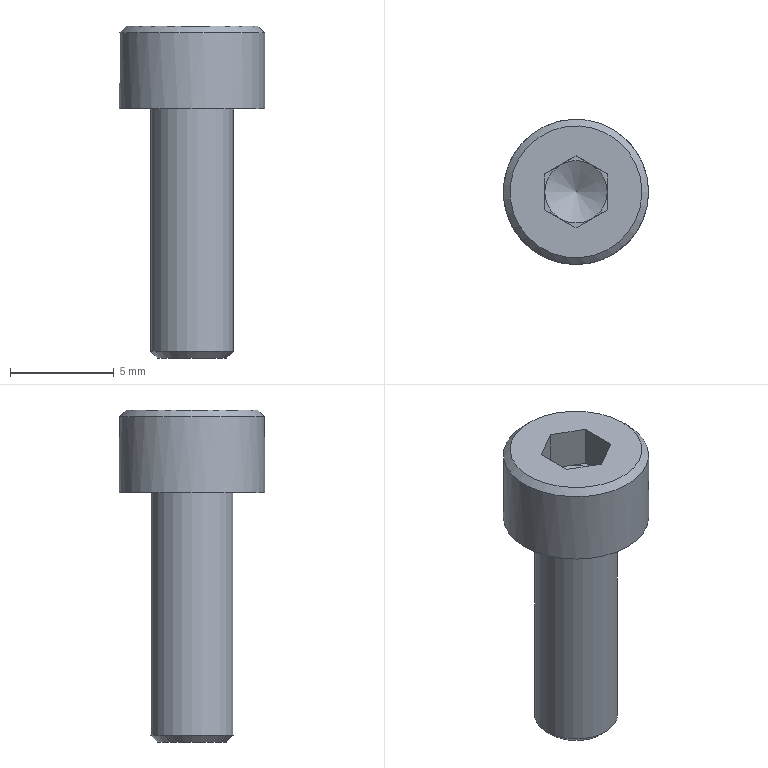Part | NX | features 切除-拉伸1 2 | 1 solid | 20 faces | box 7 x 7 x 16 mm | volume 285.405 mm3 | plane 15 | cone 3 | cylinder 2 | commonest cylinder face diameters 4 x1 7 x1
STEP:
#1=CARTESIAN_POINT('',(60.25,89.299,-85.1));
#2=VERTEX_POINT('',#1);
#3=CARTESIAN_POINT('',(59.5,88.,-85.1));
#4=VERTEX_POINT('',#3);
#5=CARTESIAN_POINT('',(61.,88.,-85.1));
#6=DIRECTION('',(0.,0.,1.));
#7=DIRECTION('',(-1.,0.,0.));
#8=AXIS2_PLACEMENT_3D('',#5,#6,#7);
#9=CIRCLE('',#8,1.5);
#10=EDGE_CURVE('',#2,#4,#9,.T.);
#11=ORIENTED_EDGE('',*,*,#10,.T.);
#12=CARTESIAN_POINT('',(60.25,86.701,-85.1));
#13=VERTEX_POINT('',#12);
#14=CARTESIAN_POINT('',(61.,88.,-85.1));
#15=DIRECTION('',(0.,0.,1.));
#16=DIRECTION('',(-1.,0.,0.));
#17=AXIS2_PLACEMENT_3D('',#14,#15,#16);
#18=CIRCLE('',#17,1.5);
#19=EDGE_CURVE('',#4,#13,#18,.T.);
#20=ORIENTED_EDGE('',*,*,#19,.T.);
#21=CARTESIAN_POINT('',(61.75,86.701,-85.1));
#22=VERTEX_POINT('',#21);
#23=CARTESIAN_POINT('',(61.,88.,-85.1));
#24=DIRECTION('',(0.,0.,1.));
#25=DIRECTION('',(-1.,0.,0.));
#26=AXIS2_PLACEMENT_3D('',#23,#24,#25);
#27=CIRCLE('',#26,1.5);
#28=EDGE_CURVE('',#13,#22,#27,.T.);
#29=ORIENTED_EDGE('',*,*,#28,.T.);
#30=CARTESIAN_POINT('',(62.5,88.,-85.1));
#31=VERTEX_POINT('',#30);
#32=CARTESIAN_POINT('',(61.,88.,-85.1));
#33=DIRECTION('',(0.,0.,1.));
#34=DIRECTION('',(-1.,0.,0.));
#35=AXIS2_PLACEMENT_3D('',#32,#33,#34);
#36=CIRCLE('',#35,1.5);
#37=EDGE_CURVE('',#22,#31,#36,.T.);
#38=ORIENTED_EDGE('',*,*,#37,.T.);
#39=CARTESIAN_POINT('',(61.75,89.299,-85.1));
#40=VERTEX_POINT('',#39);
#41=CARTESIAN_POINT('',(61.,88.,-85.1));
#42=DIRECTION('',(0.,0.,1.));
#43=DIRECTION('',(-1.,0.,0.));
#44=AXIS2_PLACEMENT_3D('',#41,#42,#43);
#45=CIRCLE('',#44,1.5);
#46=EDGE_CURVE('',#31,#40,#45,.T.);
#47=ORIENTED_EDGE('',*,*,#46,.T.);
#48=CARTESIAN_POINT('',(61.,88.,-85.1));
#49=DIRECTION('',(0.,0.,1.));
#50=DIRECTION('',(-1.,0.,0.));
#51=AXIS2_PLACEMENT_3D('',#48,#49,#50);
#52=CIRCLE('',#51,1.5);
#53=EDGE_CURVE('',#40,#2,#52,.T.);
#54=ORIENTED_EDGE('',*,*,#53,.T.);
#55=EDGE_LOOP('',(#11,#20,#29,#38,#47,#54));
#56=FACE_BOUND('',#55,.T.);
#57=CARTESIAN_POINT('',(61.,88.,-85.966));
#58=VERTEX_POINT('',#57);
#59=VERTEX_LOOP('',#58);
#60=FACE_BOUND('',#59,.T.);
#61=CARTESIAN_POINT('',(61.,88.,-85.1));
#62=DIRECTION('',(0.,0.,1.));
#63=DIRECTION('',(1.,0.,0.));
#64=AXIS2_PLACEMENT_3D('',#61,#62,#63);
#65=CONICAL_SURFACE('',#64,1.5,1.047);
#66=ADVANCED_FACE('',(#56,#60),#65,.F.);
#67=CARTESIAN_POINT('',(64.5,88.,-83.42));
#68=VERTEX_POINT('',#67);
#69=CARTESIAN_POINT('',(61.,88.,-83.42));
#70=DIRECTION('',(0.,0.,-1.));
#71=DIRECTION('',(1.,0.,0.));
#72=AXIS2_PLACEMENT_3D('',#69,#70,#71);
#73=CIRCLE('',#72,3.5);
#74=EDGE_CURVE('',#68,#68,#73,.T.);
#75=ORIENTED_EDGE('',*,*,#74,.F.);
#76=EDGE_LOOP('',(#75));
#77=FACE_BOUND('',#76,.T.);
#78=CARTESIAN_POINT('',(64.18,88.,-83.1));
#79=VERTEX_POINT('',#78);
#80=CARTESIAN_POINT('',(61.,88.,-83.1));
#81=DIRECTION('',(0.,0.,1.));
#82=DIRECTION('',(1.,0.,0.));
#83=AXIS2_PLACEMENT_3D('',#80,#81,#82);
#84=CIRCLE('',#83,3.18);
#85=EDGE_CURVE('',#79,#79,#84,.T.);
#86=ORIENTED_EDGE('',*,*,#85,.F.);
#87=EDGE_LOOP('',(#86));
#88=FACE_BOUND('',#87,.T.);
#89=CARTESIAN_POINT('',(61.,88.,-83.1));
#90=DIRECTION('',(0.,0.,-1.));
#91=DIRECTION('',(-1.,0.,0.));
#92=AXIS2_PLACEMENT_3D('',#89,#90,#91);
#93=CONICAL_SURFACE('',#92,3.18,0.7854);
#94=ADVANCED_FACE('',(#77,#88),#93,.T.);
#95=CARTESIAN_POINT('',(59.,88.,-98.78));
#96=VERTEX_POINT('',#95);
#97=CARTESIAN_POINT('',(61.,88.,-98.78));
#98=DIRECTION('',(0.,0.,1.));
#99=DIRECTION('',(-1.,0.,0.));
#100=AXIS2_PLACEMENT_3D('',#97,#98,#99);
#101=CIRCLE('',#100,2.);
#102=EDGE_CURVE('',#96,#96,#101,.T.);
#103=ORIENTED_EDGE('',*,*,#102,.F.);
#104=EDGE_LOOP('',(#103));
#105=FACE_BOUND('',#104,.T.);
#106=CARTESIAN_POINT('',(59.32,88.,-99.1));
#107=VERTEX_POINT('',#106);
#108=CARTESIAN_POINT('',(61.,88.,-99.1));
#109=DIRECTION('',(0.,0.,-1.));
#110=DIRECTION('',(-1.,0.,0.));
#111=AXIS2_PLACEMENT_3D('',#108,#109,#110);
#112=CIRCLE('',#111,1.68);
#113=EDGE_CURVE('',#107,#107,#112,.T.);
#114=ORIENTED_EDGE('',*,*,#113,.F.);
#115=EDGE_LOOP('',(#114));
#116=FACE_BOUND('',#115,.T.);
#117=CARTESIAN_POINT('',(61.,88.,-98.78));
#118=DIRECTION('',(0.,0.,1.));
#119=DIRECTION('',(1.,0.,0.));
#120=AXIS2_PLACEMENT_3D('',#117,#118,#119);
#121=CONICAL_SURFACE('',#120,2.,0.7854);
#122=ADVANCED_FACE('',(#105,#116),#121,.T.);
#123=CARTESIAN_POINT('',(59.,88.,-87.1));
#124=VERTEX_POINT('',#123);
#125=CARTESIAN_POINT('',(61.,88.,-87.1));
#126=DIRECTION('',(0.,0.,1.));
#127=DIRECTION('',(-1.,0.,0.));
#128=AXIS2_PLACEMENT_3D('',#125,#126,#127);
#129=CIRCLE('',#128,2.);
#130=EDGE_CURVE('',#124,#124,#129,.T.);
#131=ORIENTED_EDGE('',*,*,#130,.F.);
#132=EDGE_LOOP('',(#131));
#133=FACE_BOUND('',#132,.T.);
#134=ORIENTED_EDGE('',*,*,#102,.T.);
#135=EDGE_LOOP('',(#134));
#136=FACE_BOUND('',#135,.T.);
#137=CARTESIAN_POINT('',(61.,88.,-79.35));
#138=DIRECTION('',(0.,0.,1.));
#139=DIRECTION('',(1.,0.,0.));
#140=AXIS2_PLACEMENT_3D('',#137,#138,#139);
#141=CYLINDRICAL_SURFACE('',#140,2.);
#142=ADVANCED_FACE('',(#133,#136),#141,.T.);
#143=ORIENTED_EDGE('',*,*,#74,.T.);
#144=EDGE_LOOP('',(#143));
#145=FACE_BOUND('',#144,.T.);
#146=CARTESIAN_POINT('',(57.5,88.,-87.1));
#147=VERTEX_POINT('',#146);
#148=CARTESIAN_POINT('',(61.,88.,-87.1));
#149=DIRECTION('',(0.,0.,1.));
#150=DIRECTION('',(-1.,0.,0.));
#151=AXIS2_PLACEMENT_3D('',#148,#149,#150);
#152=CIRCLE('',#151,3.5);
#153=EDGE_CURVE('',#147,#147,#152,.T.);
#154=ORIENTED_EDGE('',*,*,#153,.T.);
#155=EDGE_LOOP('',(#154));
#156=FACE_BOUND('',#155,.T.);
#157=CARTESIAN_POINT('',(61.,88.,-79.35));
#158=DIRECTION('',(0.,0.,1.));
#159=DIRECTION('',(1.,0.,0.));
#160=AXIS2_PLACEMENT_3D('',#157,#158,#159);
#161=CYLINDRICAL_SURFACE('',#160,3.5);
#162=ADVANCED_FACE('',(#145,#156),#161,.T.);
#163=ORIENTED_EDGE('',*,*,#85,.T.);
#164=EDGE_LOOP('',(#163));
#165=FACE_BOUND('',#164,.T.);
#166=CARTESIAN_POINT('',(62.5,87.134,-83.1));
#167=VERTEX_POINT('',#166);
#168=CARTESIAN_POINT('',(61.,86.268,-83.1));
#169=VERTEX_POINT('',#168);
#170=CARTESIAN_POINT('',(62.875,87.35,-83.1));
#171=DIRECTION('',(-0.866,-0.5,0.));
#172=VECTOR('',#171,1000.);
#173=LINE('',#170,#172);
#174=EDGE_CURVE('',#167,#169,#173,.T.);
#175=ORIENTED_EDGE('',*,*,#174,.T.);
#176=CARTESIAN_POINT('',(59.5,87.134,-83.1));
#177=VERTEX_POINT('',#176);
#178=CARTESIAN_POINT('',(61.375,86.051,-83.1));
#179=DIRECTION('',(-0.866,0.5,0.));
#180=VECTOR('',#179,1000.);
#181=LINE('',#178,#180);
#182=EDGE_CURVE('',#169,#177,#181,.T.);
#183=ORIENTED_EDGE('',*,*,#182,.T.);
#184=CARTESIAN_POINT('',(59.5,88.866,-83.1));
#185=VERTEX_POINT('',#184);
#186=CARTESIAN_POINT('',(59.5,88.,-83.1));
#187=DIRECTION('',(0.,1.,0.));
#188=VECTOR('',#187,1000.);
#189=LINE('',#186,#188);
#190=EDGE_CURVE('',#177,#185,#189,.T.);
#191=ORIENTED_EDGE('',*,*,#190,.T.);
#192=CARTESIAN_POINT('',(61.,89.732,-83.1));
#193=VERTEX_POINT('',#192);
#194=CARTESIAN_POINT('',(61.375,89.949,-83.1));
#195=DIRECTION('',(0.866,0.5,0.));
#196=VECTOR('',#195,1000.);
#197=LINE('',#194,#196);
#198=EDGE_CURVE('',#185,#193,#197,.T.);
#199=ORIENTED_EDGE('',*,*,#198,.T.);
#200=CARTESIAN_POINT('',(62.5,88.866,-83.1));
#201=VERTEX_POINT('',#200);
#202=CARTESIAN_POINT('',(62.875,88.65,-83.1));
#203=DIRECTION('',(0.866,-0.5,0.));
#204=VECTOR('',#203,1000.);
#205=LINE('',#202,#204);
#206=EDGE_CURVE('',#193,#201,#205,.T.);
#207=ORIENTED_EDGE('',*,*,#206,.T.);
#208=CARTESIAN_POINT('',(62.5,88.,-83.1));
#209=DIRECTION('',(0.,-1.,0.));
#210=VECTOR('',#209,1000.);
#211=LINE('',#208,#210);
#212=EDGE_CURVE('',#201,#167,#211,.T.);
#213=ORIENTED_EDGE('',*,*,#212,.T.);
#214=EDGE_LOOP('',(#175,#183,#191,#199,#207,#213));
#215=FACE_BOUND('',#214,.T.);
#216=CARTESIAN_POINT('',(62.5,88.,-83.1));
#217=DIRECTION('',(0.,0.,-1.));
#218=DIRECTION('',(-1.,0.,0.));
#219=AXIS2_PLACEMENT_3D('',#216,#217,#218);
#220=PLANE('',#219);
#221=ADVANCED_FACE('',(#165,#215),#220,.F.);
#222=ORIENTED_EDGE('',*,*,#153,.F.);
#223=EDGE_LOOP('',(#222));
#224=FACE_BOUND('',#223,.T.);
#225=ORIENTED_EDGE('',*,*,#130,.T.);
#226=EDGE_LOOP('',(#225));
#227=FACE_BOUND('',#226,.T.);
#228=CARTESIAN_POINT('',(64.5,88.,-87.1));
#229=DIRECTION('',(0.,0.,1.));
#230=DIRECTION('',(1.,0.,0.));
#231=AXIS2_PLACEMENT_3D('',#228,#229,#230);
#232=PLANE('',#231);
#233=ADVANCED_FACE('',(#224,#227),#232,.F.);
#234=ORIENTED_EDGE('',*,*,#113,.T.);
#235=EDGE_LOOP('',(#234));
#236=FACE_BOUND('',#235,.T.);
#237=CARTESIAN_POINT('',(63.,88.,-99.1));
#238=DIRECTION('',(0.,0.,1.));
#239=DIRECTION('',(1.,0.,0.));
#240=AXIS2_PLACEMENT_3D('',#237,#238,#239);
#241=PLANE('',#240);
#242=ADVANCED_FACE('',(#236),#241,.F.);
#243=ORIENTED_EDGE('',*,*,#19,.F.);
#244=CARTESIAN_POINT('',(59.5,87.134,-85.1));
#245=VERTEX_POINT('',#244);
#246=CARTESIAN_POINT('',(59.5,88.866,-85.1));
#247=DIRECTION('',(0.,-1.,0.));
#248=VECTOR('',#247,1000.);
#249=LINE('',#246,#248);
#250=EDGE_CURVE('',#4,#245,#249,.T.);
#251=ORIENTED_EDGE('',*,*,#250,.T.);
#252=CARTESIAN_POINT('',(59.5,87.134,-85.1));
#253=DIRECTION('',(0.866,-0.5,0.));
#254=VECTOR('',#253,1000.);
#255=LINE('',#252,#254);
#256=EDGE_CURVE('',#245,#13,#255,.T.);
#257=ORIENTED_EDGE('',*,*,#256,.T.);
#258=EDGE_LOOP('',(#243,#251,#257));
#259=FACE_BOUND('',#258,.T.);
#260=CARTESIAN_POINT('',(61.,88.,-85.1));
#261=DIRECTION('',(0.,0.,1.));
#262=DIRECTION('',(0.,1.,0.));
#263=AXIS2_PLACEMENT_3D('',#260,#261,#262);
#264=PLANE('',#263);
#265=ADVANCED_FACE('',(#259),#264,.T.);
#266=ORIENTED_EDGE('',*,*,#10,.F.);
#267=CARTESIAN_POINT('',(59.5,88.866,-85.1));
#268=VERTEX_POINT('',#267);
#269=CARTESIAN_POINT('',(61.,89.732,-85.1));
#270=DIRECTION('',(-0.866,-0.5,0.));
#271=VECTOR('',#270,1000.);
#272=LINE('',#269,#271);
#273=EDGE_CURVE('',#2,#268,#272,.T.);
#274=ORIENTED_EDGE('',*,*,#273,.T.);
#275=CARTESIAN_POINT('',(59.5,88.866,-85.1));
#276=DIRECTION('',(0.,-1.,0.));
#277=VECTOR('',#276,1000.);
#278=LINE('',#275,#277);
#279=EDGE_CURVE('',#268,#4,#278,.T.);
#280=ORIENTED_EDGE('',*,*,#279,.T.);
#281=EDGE_LOOP('',(#266,#274,#280));
#282=FACE_BOUND('',#281,.T.);
#283=CARTESIAN_POINT('',(61.,88.,-85.1));
#284=DIRECTION('',(0.,0.,1.));
#285=DIRECTION('',(0.,1.,0.));
#286=AXIS2_PLACEMENT_3D('',#283,#284,#285);
#287=PLANE('',#286);
#288=ADVANCED_FACE('',(#282),#287,.T.);
#289=ORIENTED_EDGE('',*,*,#53,.F.);
#290=CARTESIAN_POINT('',(61.,89.732,-85.1));
#291=VERTEX_POINT('',#290);
#292=CARTESIAN_POINT('',(62.5,88.866,-85.1));
#293=DIRECTION('',(-0.866,0.5,0.));
#294=VECTOR('',#293,1000.);
#295=LINE('',#292,#294);
#296=EDGE_CURVE('',#40,#291,#295,.T.);
#297=ORIENTED_EDGE('',*,*,#296,.T.);
#298=CARTESIAN_POINT('',(61.,89.732,-85.1));
#299=DIRECTION('',(-0.866,-0.5,0.));
#300=VECTOR('',#299,1000.);
#301=LINE('',#298,#300);
#302=EDGE_CURVE('',#291,#2,#301,.T.);
#303=ORIENTED_EDGE('',*,*,#302,.T.);
#304=EDGE_LOOP('',(#289,#297,#303));
#305=FACE_BOUND('',#304,.T.);
#306=CARTESIAN_POINT('',(61.,88.,-85.1));
#307=DIRECTION('',(0.,0.,1.));
#308=DIRECTION('',(0.,1.,0.));
#309=AXIS2_PLACEMENT_3D('',#306,#307,#308);
#310=PLANE('',#309);
#311=ADVANCED_FACE('',(#305),#310,.T.);
#312=ORIENTED_EDGE('',*,*,#46,.F.);
#313=CARTESIAN_POINT('',(62.5,88.866,-85.1));
#314=VERTEX_POINT('',#313);
#315=CARTESIAN_POINT('',(62.5,87.134,-85.1));
#316=DIRECTION('',(0.,1.,0.));
#317=VECTOR('',#316,1000.);
#318=LINE('',#315,#317);
#319=EDGE_CURVE('',#31,#314,#318,.T.);
#320=ORIENTED_EDGE('',*,*,#319,.T.);
#321=CARTESIAN_POINT('',(62.5,88.866,-85.1));
#322=DIRECTION('',(-0.866,0.5,0.));
#323=VECTOR('',#322,1000.);
#324=LINE('',#321,#323);
#325=EDGE_CURVE('',#314,#40,#324,.T.);
#326=ORIENTED_EDGE('',*,*,#325,.T.);
#327=EDGE_LOOP('',(#312,#320,#326));
#328=FACE_BOUND('',#327,.T.);
#329=CARTESIAN_POINT('',(61.,88.,-85.1));
#330=DIRECTION('',(0.,0.,1.));
#331=DIRECTION('',(0.,1.,0.));
#332=AXIS2_PLACEMENT_3D('',#329,#330,#331);
#333=PLANE('',#332);
#334=ADVANCED_FACE('',(#328),#333,.T.);
#335=ORIENTED_EDGE('',*,*,#37,.F.);
#336=CARTESIAN_POINT('',(62.5,87.134,-85.1));
#337=VERTEX_POINT('',#336);
#338=CARTESIAN_POINT('',(61.,86.268,-85.1));
#339=DIRECTION('',(0.866,0.5,0.));
#340=VECTOR('',#339,1000.);
#341=LINE('',#338,#340);
#342=EDGE_CURVE('',#22,#337,#341,.T.);
#343=ORIENTED_EDGE('',*,*,#342,.T.);
#344=CARTESIAN_POINT('',(62.5,87.134,-85.1));
#345=DIRECTION('',(0.,1.,0.));
#346=VECTOR('',#345,1000.);
#347=LINE('',#344,#346);
#348=EDGE_CURVE('',#337,#31,#347,.T.);
#349=ORIENTED_EDGE('',*,*,#348,.T.);
#350=EDGE_LOOP('',(#335,#343,#349));
#351=FACE_BOUND('',#350,.T.);
#352=CARTESIAN_POINT('',(61.,88.,-85.1));
#353=DIRECTION('',(0.,0.,1.));
#354=DIRECTION('',(0.,1.,0.));
#355=AXIS2_PLACEMENT_3D('',#352,#353,#354);
#356=PLANE('',#355);
#357=ADVANCED_FACE('',(#351),#356,.T.);
#358=ORIENTED_EDGE('',*,*,#28,.F.);
#359=CARTESIAN_POINT('',(61.,86.268,-85.1));
#360=VERTEX_POINT('',#359);
#361=CARTESIAN_POINT('',(59.5,87.134,-85.1));
#362=DIRECTION('',(0.866,-0.5,0.));
#363=VECTOR('',#362,1000.);
#364=LINE('',#361,#363);
#365=EDGE_CURVE('',#13,#360,#364,.T.);
#366=ORIENTED_EDGE('',*,*,#365,.T.);
#367=CARTESIAN_POINT('',(61.,86.268,-85.1));
#368=DIRECTION('',(0.866,0.5,0.));
#369=VECTOR('',#368,1000.);
#370=LINE('',#367,#369);
#371=EDGE_CURVE('',#360,#22,#370,.T.);
#372=ORIENTED_EDGE('',*,*,#371,.T.);
#373=EDGE_LOOP('',(#358,#366,#372));
#374=FACE_BOUND('',#373,.T.);
#375=CARTESIAN_POINT('',(61.,88.,-85.1));
#376=DIRECTION('',(0.,0.,1.));
#377=DIRECTION('',(0.,1.,0.));
#378=AXIS2_PLACEMENT_3D('',#375,#376,#377);
#379=PLANE('',#378);
#380=ADVANCED_FACE('',(#374),#379,.T.);
#381=ORIENTED_EDGE('',*,*,#182,.F.);
#382=CARTESIAN_POINT('',(61.,86.268,-85.1));
#383=DIRECTION('',(0.,0.,1.));
#384=VECTOR('',#383,1000.);
#385=LINE('',#382,#384);
#386=EDGE_CURVE('',#360,#169,#385,.T.);
#387=ORIENTED_EDGE('',*,*,#386,.F.);
#388=ORIENTED_EDGE('',*,*,#365,.F.);
#389=ORIENTED_EDGE('',*,*,#256,.F.);
#390=CARTESIAN_POINT('',(59.5,87.134,-85.1));
#391=DIRECTION('',(0.,0.,1.));
#392=VECTOR('',#391,1000.);
#393=LINE('',#390,#392);
#394=EDGE_CURVE('',#245,#177,#393,.T.);
#395=ORIENTED_EDGE('',*,*,#394,.T.);
#396=EDGE_LOOP('',(#381,#387,#388,#389,#395));
#397=FACE_BOUND('',#396,.T.);
#398=CARTESIAN_POINT('',(59.5,87.134,-85.1));
#399=DIRECTION('',(-0.5,-0.866,0.));
#400=DIRECTION('',(0.866,-0.5,0.));
#401=AXIS2_PLACEMENT_3D('',#398,#399,#400);
#402=PLANE('',#401);
#403=ADVANCED_FACE('',(#397),#402,.F.);
#404=ORIENTED_EDGE('',*,*,#190,.F.);
#405=ORIENTED_EDGE('',*,*,#394,.F.);
#406=ORIENTED_EDGE('',*,*,#250,.F.);
#407=ORIENTED_EDGE('',*,*,#279,.F.);
#408=CARTESIAN_POINT('',(59.5,88.866,-85.1));
#409=DIRECTION('',(0.,0.,1.));
#410=VECTOR('',#409,1000.);
#411=LINE('',#408,#410);
#412=EDGE_CURVE('',#268,#185,#411,.T.);
#413=ORIENTED_EDGE('',*,*,#412,.T.);
#414=EDGE_LOOP('',(#404,#405,#406,#407,#413));
#415=FACE_BOUND('',#414,.T.);
#416=CARTESIAN_POINT('',(59.5,88.866,-85.1));
#417=DIRECTION('',(-1.,0.,0.));
#418=DIRECTION('',(0.,0.,1.));
#419=AXIS2_PLACEMENT_3D('',#416,#417,#418);
#420=PLANE('',#419);
#421=ADVANCED_FACE('',(#415),#420,.F.);
#422=ORIENTED_EDGE('',*,*,#198,.F.);
#423=ORIENTED_EDGE('',*,*,#412,.F.);
#424=ORIENTED_EDGE('',*,*,#273,.F.);
#425=ORIENTED_EDGE('',*,*,#302,.F.);
#426=CARTESIAN_POINT('',(61.,89.732,-85.1));
#427=DIRECTION('',(0.,0.,1.));
#428=VECTOR('',#427,1000.);
#429=LINE('',#426,#428);
#430=EDGE_CURVE('',#291,#193,#429,.T.);
#431=ORIENTED_EDGE('',*,*,#430,.T.);
#432=EDGE_LOOP('',(#422,#423,#424,#425,#431));
#433=FACE_BOUND('',#432,.T.);
#434=CARTESIAN_POINT('',(61.,89.732,-85.1));
#435=DIRECTION('',(-0.5,0.866,0.));
#436=DIRECTION('',(-0.866,-0.5,0.));
#437=AXIS2_PLACEMENT_3D('',#434,#435,#436);
#438=PLANE('',#437);
#439=ADVANCED_FACE('',(#433),#438,.F.);
#440=ORIENTED_EDGE('',*,*,#206,.F.);
#441=ORIENTED_EDGE('',*,*,#430,.F.);
#442=ORIENTED_EDGE('',*,*,#296,.F.);
#443=ORIENTED_EDGE('',*,*,#325,.F.);
#444=CARTESIAN_POINT('',(62.5,88.866,-85.1));
#445=DIRECTION('',(0.,0.,1.));
#446=VECTOR('',#445,1000.);
#447=LINE('',#444,#446);
#448=EDGE_CURVE('',#314,#201,#447,.T.);
#449=ORIENTED_EDGE('',*,*,#448,.T.);
#450=EDGE_LOOP('',(#440,#441,#442,#443,#449));
#451=FACE_BOUND('',#450,.T.);
#452=CARTESIAN_POINT('',(62.5,88.866,-85.1));
#453=DIRECTION('',(0.5,0.866,0.));
#454=DIRECTION('',(-0.866,0.5,0.));
#455=AXIS2_PLACEMENT_3D('',#452,#453,#454);
#456=PLANE('',#455);
#457=ADVANCED_FACE('',(#451),#456,.F.);
#458=ORIENTED_EDGE('',*,*,#212,.F.);
#459=ORIENTED_EDGE('',*,*,#448,.F.);
#460=ORIENTED_EDGE('',*,*,#319,.F.);
#461=ORIENTED_EDGE('',*,*,#348,.F.);
#462=CARTESIAN_POINT('',(62.5,87.134,-85.1));
#463=DIRECTION('',(0.,0.,1.));
#464=VECTOR('',#463,1000.);
#465=LINE('',#462,#464);
#466=EDGE_CURVE('',#337,#167,#465,.T.);
#467=ORIENTED_EDGE('',*,*,#466,.T.);
#468=EDGE_LOOP('',(#458,#459,#460,#461,#467));
#469=FACE_BOUND('',#468,.T.);
#470=CARTESIAN_POINT('',(62.5,87.134,-85.1));
#471=DIRECTION('',(1.,0.,0.));
#472=DIRECTION('',(0.,0.,-1.));
#473=AXIS2_PLACEMENT_3D('',#470,#471,#472);
#474=PLANE('',#473);
#475=ADVANCED_FACE('',(#469),#474,.F.);
#476=ORIENTED_EDGE('',*,*,#174,.F.);
#477=ORIENTED_EDGE('',*,*,#466,.F.);
#478=ORIENTED_EDGE('',*,*,#342,.F.);
#479=ORIENTED_EDGE('',*,*,#371,.F.);
#480=ORIENTED_EDGE('',*,*,#386,.T.);
#481=EDGE_LOOP('',(#476,#477,#478,#479,#480));
#482=FACE_BOUND('',#481,.T.);
#483=CARTESIAN_POINT('',(61.,86.268,-85.1));
#484=DIRECTION('',(0.5,-0.866,0.));
#485=DIRECTION('',(0.866,0.5,0.));
#486=AXIS2_PLACEMENT_3D('',#483,#484,#485);
#487=PLANE('',#486);
#488=ADVANCED_FACE('',(#482),#487,.F.);
#489=CLOSED_SHELL('',(#66,#94,#122,#142,#162,#221,#233,#242,#265,#288,#311,#334,#357,#380,#403,#421,#439,#457,#475,#488));
#490=MANIFOLD_SOLID_BREP('',#489);
#491=(LENGTH_UNIT()NAMED_UNIT(*)SI_UNIT(.MILLI.,.METRE.));
#492=UNCERTAINTY_MEASURE_WITH_UNIT(LENGTH_MEASURE(0.00001),#491,'','');
#493=(NAMED_UNIT(*)PLANE_ANGLE_UNIT()SI_UNIT($,.RADIAN.));
#494=(NAMED_UNIT(*)SI_UNIT($,.STERADIAN.)SOLID_ANGLE_UNIT());
#495=(GEOMETRIC_REPRESENTATION_CONTEXT(3)GLOBAL_UNCERTAINTY_ASSIGNED_CONTEXT((#492))GLOBAL_UNIT_ASSIGNED_CONTEXT((#491,#493,#494))REPRESENTATION_CONTEXT('',''));
#496=ADVANCED_BREP_SHAPE_REPRESENTATION('',(#490),#495);